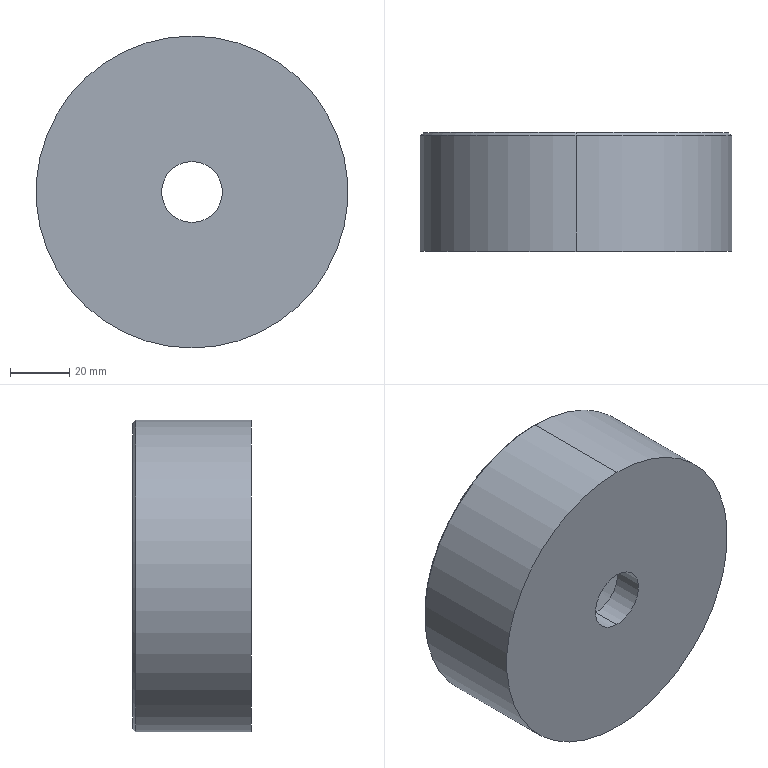Part | SolidWorks | features BaseBody 1 | 1 solid | 13 faces | box 105 x 40 x 105 mm | volume 172526 mm3 | cylinder 6 | cone 4 | plane 3 | commonest cylinder face diameters 20.5 x2 85 x2 105 x2
STEP:
#1=CARTESIAN_POINT('',(0.,39.,-52.5));
#2=VERTEX_POINT('',#1);
#3=CARTESIAN_POINT('',(0.,39.,52.5));
#4=VERTEX_POINT('',#3);
#5=CARTESIAN_POINT('',(0.,39.,0.));
#6=DIRECTION('',(0.,-1.,0.));
#7=DIRECTION('',(0.,0.,-1.));
#8=AXIS2_PLACEMENT_3D('',#5,#6,#7);
#9=CIRCLE('',#8,52.5);
#10=EDGE_CURVE('',#2,#4,#9,.T.);
#11=ORIENTED_EDGE('',*,*,#10,.T.);
#12=CARTESIAN_POINT('',(0.,0.,52.5));
#13=VERTEX_POINT('',#12);
#14=CARTESIAN_POINT('',(0.,40.,52.5));
#15=DIRECTION('',(0.,-1.,0.));
#16=VECTOR('',#15,1000.);
#17=LINE('',#14,#16);
#18=EDGE_CURVE('',#4,#13,#17,.T.);
#19=ORIENTED_EDGE('',*,*,#18,.T.);
#20=CARTESIAN_POINT('',(0.,0.,-52.5));
#21=VERTEX_POINT('',#20);
#22=CARTESIAN_POINT('',(0.,0.,0.));
#23=DIRECTION('',(0.,1.,0.));
#24=DIRECTION('',(0.,0.,-1.));
#25=AXIS2_PLACEMENT_3D('',#22,#23,#24);
#26=CIRCLE('',#25,52.5);
#27=EDGE_CURVE('',#13,#21,#26,.T.);
#28=ORIENTED_EDGE('',*,*,#27,.T.);
#29=CARTESIAN_POINT('',(0.,40.,-52.5));
#30=DIRECTION('',(0.,-1.,0.));
#31=VECTOR('',#30,1000.);
#32=LINE('',#29,#31);
#33=EDGE_CURVE('',#2,#21,#32,.T.);
#34=ORIENTED_EDGE('',*,*,#33,.F.);
#35=EDGE_LOOP('',(#11,#19,#28,#34));
#36=FACE_OUTER_BOUND('',#35,.T.);
#37=CARTESIAN_POINT('',(0.,40.,0.));
#38=DIRECTION('',(0.,-1.,0.));
#39=DIRECTION('',(0.,0.,-1.));
#40=AXIS2_PLACEMENT_3D('',#37,#38,#39);
#41=CYLINDRICAL_SURFACE('',#40,52.5);
#42=ADVANCED_FACE('',(#36),#41,.T.);
#43=CARTESIAN_POINT('',(0.,0.,10.25));
#44=VERTEX_POINT('',#43);
#45=CARTESIAN_POINT('',(0.,0.,-10.25));
#46=VERTEX_POINT('',#45);
#47=CARTESIAN_POINT('',(0.,0.,0.));
#48=DIRECTION('',(0.,-1.,0.));
#49=DIRECTION('',(0.,0.,1.));
#50=AXIS2_PLACEMENT_3D('',#47,#48,#49);
#51=CIRCLE('',#50,10.25);
#52=EDGE_CURVE('',#44,#46,#51,.T.);
#53=ORIENTED_EDGE('',*,*,#52,.T.);
#54=CARTESIAN_POINT('',(0.,10.,-10.25));
#55=VERTEX_POINT('',#54);
#56=CARTESIAN_POINT('',(0.,10.,-10.25));
#57=DIRECTION('',(0.,1.,0.));
#58=VECTOR('',#57,1000.);
#59=LINE('',#56,#58);
#60=EDGE_CURVE('',#46,#55,#59,.T.);
#61=ORIENTED_EDGE('',*,*,#60,.T.);
#62=CARTESIAN_POINT('',(0.,10.,10.25));
#63=VERTEX_POINT('',#62);
#64=CARTESIAN_POINT('',(0.,10.,0.));
#65=DIRECTION('',(0.,-1.,0.));
#66=DIRECTION('',(0.,0.,1.));
#67=AXIS2_PLACEMENT_3D('',#64,#65,#66);
#68=CIRCLE('',#67,10.25);
#69=EDGE_CURVE('',#63,#55,#68,.T.);
#70=ORIENTED_EDGE('',*,*,#69,.F.);
#71=CARTESIAN_POINT('',(0.,10.,10.25));
#72=DIRECTION('',(0.,1.,0.));
#73=VECTOR('',#72,1000.);
#74=LINE('',#71,#73);
#75=EDGE_CURVE('',#44,#63,#74,.T.);
#76=ORIENTED_EDGE('',*,*,#75,.F.);
#77=EDGE_LOOP('',(#53,#61,#70,#76));
#78=FACE_OUTER_BOUND('',#77,.T.);
#79=CARTESIAN_POINT('',(0.,10.,0.));
#80=DIRECTION('',(0.,1.,0.));
#81=DIRECTION('',(0.,0.,1.));
#82=AXIS2_PLACEMENT_3D('',#79,#80,#81);
#83=CYLINDRICAL_SURFACE('',#82,10.25);
#84=ADVANCED_FACE('',(#78),#83,.F.);
#85=CARTESIAN_POINT('',(0.,40.,-51.5));
#86=VERTEX_POINT('',#85);
#87=CARTESIAN_POINT('',(0.,40.,51.5));
#88=VERTEX_POINT('',#87);
#89=CARTESIAN_POINT('',(0.,40.,0.));
#90=DIRECTION('',(0.,-1.,0.));
#91=DIRECTION('',(0.,0.,-1.));
#92=AXIS2_PLACEMENT_3D('',#89,#90,#91);
#93=CIRCLE('',#92,51.5);
#94=EDGE_CURVE('',#86,#88,#93,.T.);
#95=ORIENTED_EDGE('',*,*,#94,.T.);
#96=CARTESIAN_POINT('',(0.,39.,52.5));
#97=DIRECTION('',(0.,-0.7071,0.7071));
#98=VECTOR('',#97,1000.);
#99=LINE('',#96,#98);
#100=EDGE_CURVE('',#88,#4,#99,.T.);
#101=ORIENTED_EDGE('',*,*,#100,.T.);
#102=ORIENTED_EDGE('',*,*,#10,.F.);
#103=CARTESIAN_POINT('',(0.,39.,-52.5));
#104=DIRECTION('',(0.,-0.7071,-0.7071));
#105=VECTOR('',#104,1000.);
#106=LINE('',#103,#105);
#107=EDGE_CURVE('',#86,#2,#106,.T.);
#108=ORIENTED_EDGE('',*,*,#107,.F.);
#109=EDGE_LOOP('',(#95,#101,#102,#108));
#110=FACE_OUTER_BOUND('',#109,.T.);
#111=CARTESIAN_POINT('',(0.,39.,0.));
#112=DIRECTION('',(0.,-1.,0.));
#113=DIRECTION('',(0.,0.,-1.));
#114=AXIS2_PLACEMENT_3D('',#111,#112,#113);
#115=CONICAL_SURFACE('',#114,52.5,0.7854);
#116=ADVANCED_FACE('',(#110),#115,.T.);
#117=CARTESIAN_POINT('',(0.,10.,-42.5));
#118=VERTEX_POINT('',#117);
#119=CARTESIAN_POINT('',(0.,10.,42.5));
#120=VERTEX_POINT('',#119);
#121=CARTESIAN_POINT('',(0.,10.,0.));
#122=DIRECTION('',(0.,1.,0.));
#123=DIRECTION('',(0.,0.,1.));
#124=AXIS2_PLACEMENT_3D('',#121,#122,#123);
#125=CIRCLE('',#124,42.5);
#126=EDGE_CURVE('',#118,#120,#125,.T.);
#127=ORIENTED_EDGE('',*,*,#126,.F.);
#128=CARTESIAN_POINT('',(0.,39.,-42.5));
#129=VERTEX_POINT('',#128);
#130=CARTESIAN_POINT('',(0.,10.,-42.5));
#131=DIRECTION('',(0.,1.,0.));
#132=VECTOR('',#131,1000.);
#133=LINE('',#130,#132);
#134=EDGE_CURVE('',#118,#129,#133,.T.);
#135=ORIENTED_EDGE('',*,*,#134,.T.);
#136=CARTESIAN_POINT('',(-42.5,39.,0.));
#137=VERTEX_POINT('',#136);
#138=CARTESIAN_POINT('',(0.,39.,0.));
#139=DIRECTION('',(0.,-1.,0.));
#140=DIRECTION('',(0.,0.,1.));
#141=AXIS2_PLACEMENT_3D('',#138,#139,#140);
#142=CIRCLE('',#141,42.5);
#143=EDGE_CURVE('',#137,#129,#142,.T.);
#144=ORIENTED_EDGE('',*,*,#143,.F.);
#145=CARTESIAN_POINT('',(0.,39.,42.5));
#146=VERTEX_POINT('',#145);
#147=CARTESIAN_POINT('',(0.,39.,0.));
#148=DIRECTION('',(0.,-1.,0.));
#149=DIRECTION('',(0.,0.,1.));
#150=AXIS2_PLACEMENT_3D('',#147,#148,#149);
#151=CIRCLE('',#150,42.5);
#152=EDGE_CURVE('',#146,#137,#151,.T.);
#153=ORIENTED_EDGE('',*,*,#152,.F.);
#154=CARTESIAN_POINT('',(0.,10.,42.5));
#155=DIRECTION('',(0.,1.,0.));
#156=VECTOR('',#155,1000.);
#157=LINE('',#154,#156);
#158=EDGE_CURVE('',#120,#146,#157,.T.);
#159=ORIENTED_EDGE('',*,*,#158,.F.);
#160=EDGE_LOOP('',(#127,#135,#144,#153,#159));
#161=FACE_OUTER_BOUND('',#160,.T.);
#162=CARTESIAN_POINT('',(0.,10.,0.));
#163=DIRECTION('',(0.,1.,0.));
#164=DIRECTION('',(0.,0.,1.));
#165=AXIS2_PLACEMENT_3D('',#162,#163,#164);
#166=CYLINDRICAL_SURFACE('',#165,42.5);
#167=ADVANCED_FACE('',(#161),#166,.F.);
#168=ORIENTED_EDGE('',*,*,#143,.T.);
#169=CARTESIAN_POINT('',(42.5,39.,0.));
#170=VERTEX_POINT('',#169);
#171=CARTESIAN_POINT('',(0.,39.,0.));
#172=DIRECTION('',(0.,-1.,0.));
#173=DIRECTION('',(0.,0.,1.));
#174=AXIS2_PLACEMENT_3D('',#171,#172,#173);
#175=CIRCLE('',#174,42.5);
#176=EDGE_CURVE('',#129,#170,#175,.T.);
#177=ORIENTED_EDGE('',*,*,#176,.T.);
#178=CARTESIAN_POINT('',(43.5,40.,0.));
#179=VERTEX_POINT('',#178);
#180=CARTESIAN_POINT('',(43.5,40.,0.));
#181=DIRECTION('',(0.7071,0.7071,0.));
#182=VECTOR('',#181,1000.);
#183=LINE('',#180,#182);
#184=EDGE_CURVE('',#170,#179,#183,.T.);
#185=ORIENTED_EDGE('',*,*,#184,.T.);
#186=CARTESIAN_POINT('',(-43.5,40.,0.));
#187=VERTEX_POINT('',#186);
#188=CARTESIAN_POINT('',(0.,40.,0.));
#189=DIRECTION('',(0.,-1.,0.));
#190=DIRECTION('',(-1.,0.,0.));
#191=AXIS2_PLACEMENT_3D('',#188,#189,#190);
#192=CIRCLE('',#191,43.5);
#193=EDGE_CURVE('',#187,#179,#192,.T.);
#194=ORIENTED_EDGE('',*,*,#193,.F.);
#195=CARTESIAN_POINT('',(-43.5,40.,0.));
#196=DIRECTION('',(-0.7071,0.7071,0.));
#197=VECTOR('',#196,1000.);
#198=LINE('',#195,#197);
#199=EDGE_CURVE('',#137,#187,#198,.T.);
#200=ORIENTED_EDGE('',*,*,#199,.F.);
#201=EDGE_LOOP('',(#168,#177,#185,#194,#200));
#202=FACE_OUTER_BOUND('',#201,.T.);
#203=CARTESIAN_POINT('',(0.,40.,0.));
#204=DIRECTION('',(0.,1.,0.));
#205=DIRECTION('',(-1.,0.,0.));
#206=AXIS2_PLACEMENT_3D('',#203,#204,#205);
#207=CONICAL_SURFACE('',#206,43.5,0.7854);
#208=ADVANCED_FACE('',(#202),#207,.F.);
#209=CARTESIAN_POINT('',(0.,0.,0.));
#210=DIRECTION('',(0.,1.,0.));
#211=DIRECTION('',(0.,0.,-1.));
#212=AXIS2_PLACEMENT_3D('',#209,#210,#211);
#213=CIRCLE('',#212,52.5);
#214=EDGE_CURVE('',#21,#13,#213,.T.);
#215=ORIENTED_EDGE('',*,*,#214,.F.);
#216=ORIENTED_EDGE('',*,*,#27,.F.);
#217=EDGE_LOOP('',(#215,#216));
#218=FACE_OUTER_BOUND('',#217,.T.);
#219=ORIENTED_EDGE('',*,*,#52,.F.);
#220=CARTESIAN_POINT('',(0.,0.,0.));
#221=DIRECTION('',(0.,-1.,0.));
#222=DIRECTION('',(0.,0.,1.));
#223=AXIS2_PLACEMENT_3D('',#220,#221,#222);
#224=CIRCLE('',#223,10.25);
#225=EDGE_CURVE('',#46,#44,#224,.T.);
#226=ORIENTED_EDGE('',*,*,#225,.F.);
#227=EDGE_LOOP('',(#219,#226));
#228=FACE_BOUND('',#227,.T.);
#229=CARTESIAN_POINT('',(0.,0.,0.));
#230=DIRECTION('',(0.,1.,0.));
#231=DIRECTION('',(0.,0.,1.));
#232=AXIS2_PLACEMENT_3D('',#229,#230,#231);
#233=PLANE('',#232);
#234=ADVANCED_FACE('',(#218,#228),#233,.F.);
#235=ORIENTED_EDGE('',*,*,#18,.F.);
#236=CARTESIAN_POINT('',(0.,39.,0.));
#237=DIRECTION('',(0.,-1.,0.));
#238=DIRECTION('',(0.,0.,-1.));
#239=AXIS2_PLACEMENT_3D('',#236,#237,#238);
#240=CIRCLE('',#239,52.5);
#241=EDGE_CURVE('',#4,#2,#240,.T.);
#242=ORIENTED_EDGE('',*,*,#241,.T.);
#243=ORIENTED_EDGE('',*,*,#33,.T.);
#244=ORIENTED_EDGE('',*,*,#214,.T.);
#245=EDGE_LOOP('',(#235,#242,#243,#244));
#246=FACE_OUTER_BOUND('',#245,.T.);
#247=CARTESIAN_POINT('',(0.,40.,0.));
#248=DIRECTION('',(0.,-1.,0.));
#249=DIRECTION('',(0.,0.,-1.));
#250=AXIS2_PLACEMENT_3D('',#247,#248,#249);
#251=CYLINDRICAL_SURFACE('',#250,52.5);
#252=ADVANCED_FACE('',(#246),#251,.T.);
#253=ORIENTED_EDGE('',*,*,#60,.F.);
#254=ORIENTED_EDGE('',*,*,#225,.T.);
#255=ORIENTED_EDGE('',*,*,#75,.T.);
#256=CARTESIAN_POINT('',(0.,10.,0.));
#257=DIRECTION('',(0.,-1.,0.));
#258=DIRECTION('',(0.,0.,1.));
#259=AXIS2_PLACEMENT_3D('',#256,#257,#258);
#260=CIRCLE('',#259,10.25);
#261=EDGE_CURVE('',#55,#63,#260,.T.);
#262=ORIENTED_EDGE('',*,*,#261,.F.);
#263=EDGE_LOOP('',(#253,#254,#255,#262));
#264=FACE_OUTER_BOUND('',#263,.T.);
#265=CARTESIAN_POINT('',(0.,10.,0.));
#266=DIRECTION('',(0.,1.,0.));
#267=DIRECTION('',(0.,0.,1.));
#268=AXIS2_PLACEMENT_3D('',#265,#266,#267);
#269=CYLINDRICAL_SURFACE('',#268,10.25);
#270=ADVANCED_FACE('',(#264),#269,.F.);
#271=ORIENTED_EDGE('',*,*,#100,.F.);
#272=CARTESIAN_POINT('',(0.,40.,0.));
#273=DIRECTION('',(0.,-1.,0.));
#274=DIRECTION('',(0.,0.,-1.));
#275=AXIS2_PLACEMENT_3D('',#272,#273,#274);
#276=CIRCLE('',#275,51.5);
#277=EDGE_CURVE('',#88,#86,#276,.T.);
#278=ORIENTED_EDGE('',*,*,#277,.T.);
#279=ORIENTED_EDGE('',*,*,#107,.T.);
#280=ORIENTED_EDGE('',*,*,#241,.F.);
#281=EDGE_LOOP('',(#271,#278,#279,#280));
#282=FACE_OUTER_BOUND('',#281,.T.);
#283=CARTESIAN_POINT('',(0.,39.,0.));
#284=DIRECTION('',(0.,-1.,0.));
#285=DIRECTION('',(0.,0.,-1.));
#286=AXIS2_PLACEMENT_3D('',#283,#284,#285);
#287=CONICAL_SURFACE('',#286,52.5,0.7854);
#288=ADVANCED_FACE('',(#282),#287,.T.);
#289=CARTESIAN_POINT('',(0.,10.,0.));
#290=DIRECTION('',(0.,1.,0.));
#291=DIRECTION('',(0.,0.,1.));
#292=AXIS2_PLACEMENT_3D('',#289,#290,#291);
#293=CIRCLE('',#292,42.5);
#294=EDGE_CURVE('',#120,#118,#293,.T.);
#295=ORIENTED_EDGE('',*,*,#294,.T.);
#296=ORIENTED_EDGE('',*,*,#126,.T.);
#297=EDGE_LOOP('',(#295,#296));
#298=FACE_OUTER_BOUND('',#297,.T.);
#299=ORIENTED_EDGE('',*,*,#69,.T.);
#300=ORIENTED_EDGE('',*,*,#261,.T.);
#301=EDGE_LOOP('',(#299,#300));
#302=FACE_BOUND('',#301,.T.);
#303=CARTESIAN_POINT('',(0.,10.,0.));
#304=DIRECTION('',(0.,1.,0.));
#305=DIRECTION('',(0.,0.,1.));
#306=AXIS2_PLACEMENT_3D('',#303,#304,#305);
#307=PLANE('',#306);
#308=ADVANCED_FACE('',(#298,#302),#307,.T.);
#309=ORIENTED_EDGE('',*,*,#193,.T.);
#310=CARTESIAN_POINT('',(0.,40.,0.));
#311=DIRECTION('',(0.,-1.,0.));
#312=DIRECTION('',(-1.,0.,0.));
#313=AXIS2_PLACEMENT_3D('',#310,#311,#312);
#314=CIRCLE('',#313,43.5);
#315=EDGE_CURVE('',#179,#187,#314,.T.);
#316=ORIENTED_EDGE('',*,*,#315,.T.);
#317=EDGE_LOOP('',(#309,#316));
#318=FACE_BOUND('',#317,.T.);
#319=ORIENTED_EDGE('',*,*,#94,.F.);
#320=ORIENTED_EDGE('',*,*,#277,.F.);
#321=EDGE_LOOP('',(#319,#320));
#322=FACE_OUTER_BOUND('',#321,.T.);
#323=CARTESIAN_POINT('',(0.,40.,0.));
#324=DIRECTION('',(0.,1.,0.));
#325=DIRECTION('',(0.,0.,1.));
#326=AXIS2_PLACEMENT_3D('',#323,#324,#325);
#327=PLANE('',#326);
#328=ADVANCED_FACE('',(#318,#322),#327,.T.);
#329=ORIENTED_EDGE('',*,*,#134,.F.);
#330=ORIENTED_EDGE('',*,*,#294,.F.);
#331=ORIENTED_EDGE('',*,*,#158,.T.);
#332=CARTESIAN_POINT('',(0.,39.,0.));
#333=DIRECTION('',(0.,-1.,0.));
#334=DIRECTION('',(0.,0.,1.));
#335=AXIS2_PLACEMENT_3D('',#332,#333,#334);
#336=CIRCLE('',#335,42.5);
#337=EDGE_CURVE('',#170,#146,#336,.T.);
#338=ORIENTED_EDGE('',*,*,#337,.F.);
#339=ORIENTED_EDGE('',*,*,#176,.F.);
#340=EDGE_LOOP('',(#329,#330,#331,#338,#339));
#341=FACE_OUTER_BOUND('',#340,.T.);
#342=CARTESIAN_POINT('',(0.,10.,0.));
#343=DIRECTION('',(0.,1.,0.));
#344=DIRECTION('',(0.,0.,1.));
#345=AXIS2_PLACEMENT_3D('',#342,#343,#344);
#346=CYLINDRICAL_SURFACE('',#345,42.5);
#347=ADVANCED_FACE('',(#341),#346,.F.);
#348=ORIENTED_EDGE('',*,*,#184,.F.);
#349=ORIENTED_EDGE('',*,*,#337,.T.);
#350=ORIENTED_EDGE('',*,*,#152,.T.);
#351=ORIENTED_EDGE('',*,*,#199,.T.);
#352=ORIENTED_EDGE('',*,*,#315,.F.);
#353=EDGE_LOOP('',(#348,#349,#350,#351,#352));
#354=FACE_OUTER_BOUND('',#353,.T.);
#355=CARTESIAN_POINT('',(0.,40.,0.));
#356=DIRECTION('',(0.,1.,0.));
#357=DIRECTION('',(-1.,0.,0.));
#358=AXIS2_PLACEMENT_3D('',#355,#356,#357);
#359=CONICAL_SURFACE('',#358,43.5,0.7854);
#360=ADVANCED_FACE('',(#354),#359,.F.);
#361=CLOSED_SHELL('',(#42,#84,#116,#167,#208,#234,#252,#270,#288,#308,#328,#347,#360));
#362=MANIFOLD_SOLID_BREP('',#361);
#363=CARTESIAN_POINT('',(0.,0.,0.));
#364=DIRECTION('',(0.,0.,1.));
#365=DIRECTION('',(1.,0.,0.));
#366=AXIS2_PLACEMENT_3D('',#363,#364,#365);
#367=(LENGTH_UNIT()NAMED_UNIT(*)SI_UNIT(.MILLI.,.METRE.));
#368=UNCERTAINTY_MEASURE_WITH_UNIT(LENGTH_MEASURE(0.00001),#367,'','');
#369=(NAMED_UNIT(*)PLANE_ANGLE_UNIT()SI_UNIT($,.RADIAN.));
#370=(NAMED_UNIT(*)SI_UNIT($,.STERADIAN.)SOLID_ANGLE_UNIT());
#371=(GEOMETRIC_REPRESENTATION_CONTEXT(3)GLOBAL_UNCERTAINTY_ASSIGNED_CONTEXT((#368))GLOBAL_UNIT_ASSIGNED_CONTEXT((#367,#369,#370))REPRESENTATION_CONTEXT('',''));
#372=ADVANCED_BREP_SHAPE_REPRESENTATION('',(#362,#366),#371);